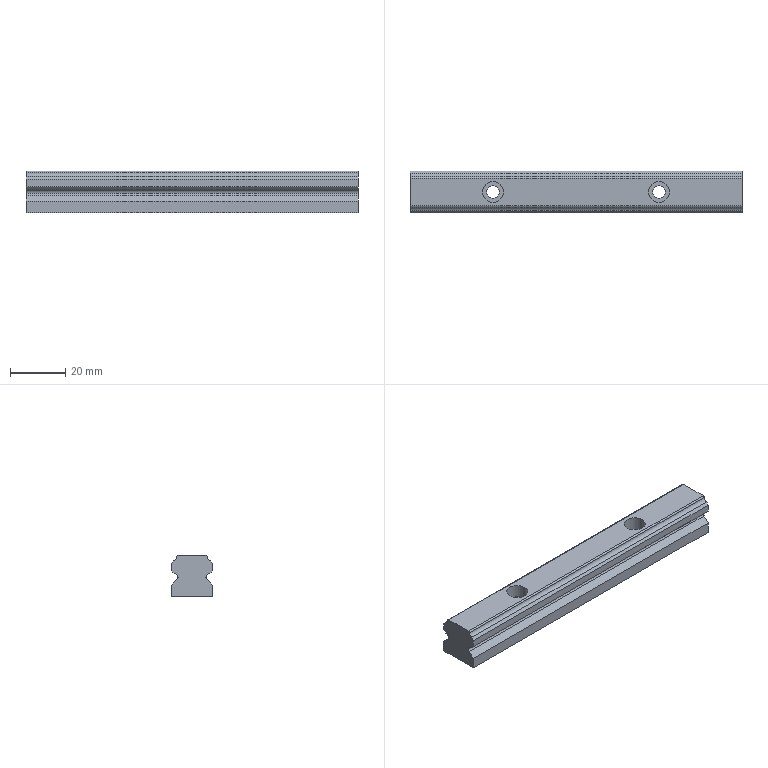Part | STEP file | Tube necking machine_id510_x_t | 1 solid | 28 faces | box 120 x 15 x 15 mm | volume 23510 mm3 | plane 16 | cylinder 12 | commonest cylinder face diameters 3 x6 1 x2 4.5 x2 7.6 x2